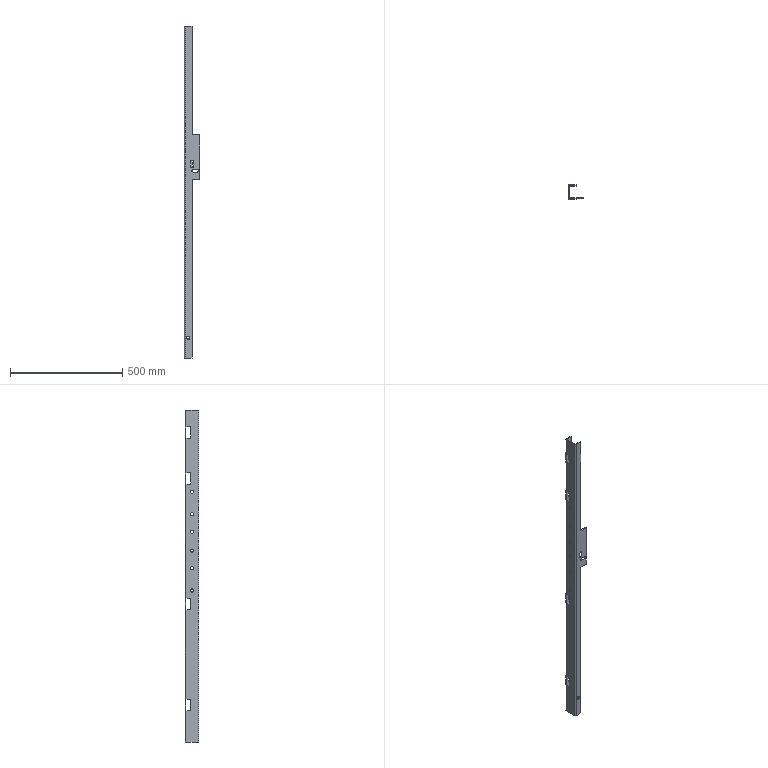Part | SolidWorks | features ICE 10, SMBaseFlange 5, Cut 1, FlatPattern 1, SheetMetal 1 | 1 solid | 129 faces | box 70 x 62 x 1480 mm | volume 721616 mm3 | plane 84 | cylinder 45 | commonest cylinder face diameters 10 x12 14.5 x12 0.4 x6 8.4 x6 12 x5 11 x2